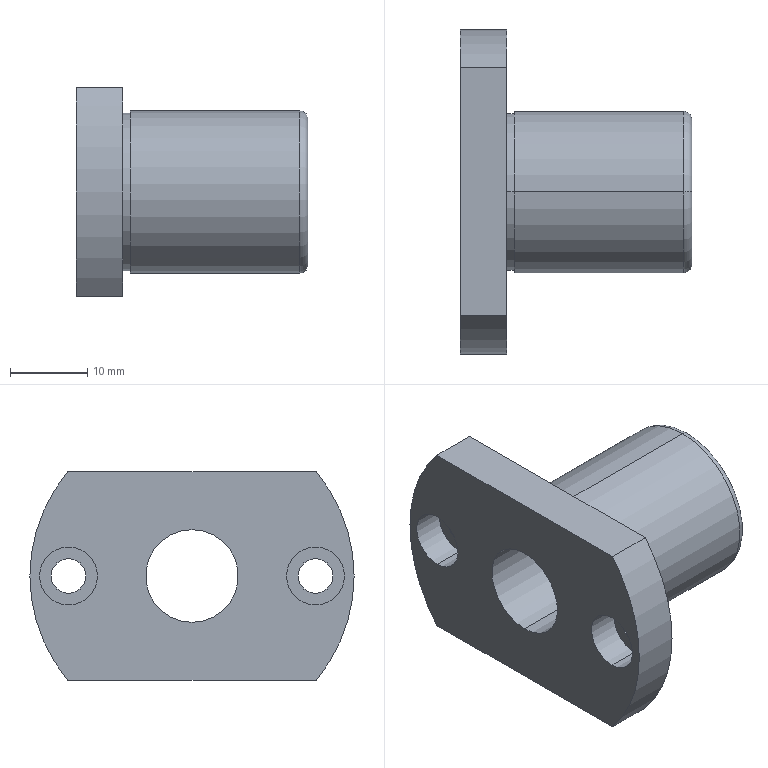Part | STEP file | LHFC12_LHFC12 | 1 solid | 26 faces | box 30 x 42 x 27 mm | volume 10763 mm3 | cylinder 16 | plane 8 | torus 2 | commonest cylinder face diameters 4.5 x4 7.5 x4 12 x2 20.4 x2 21 x2 42 x2